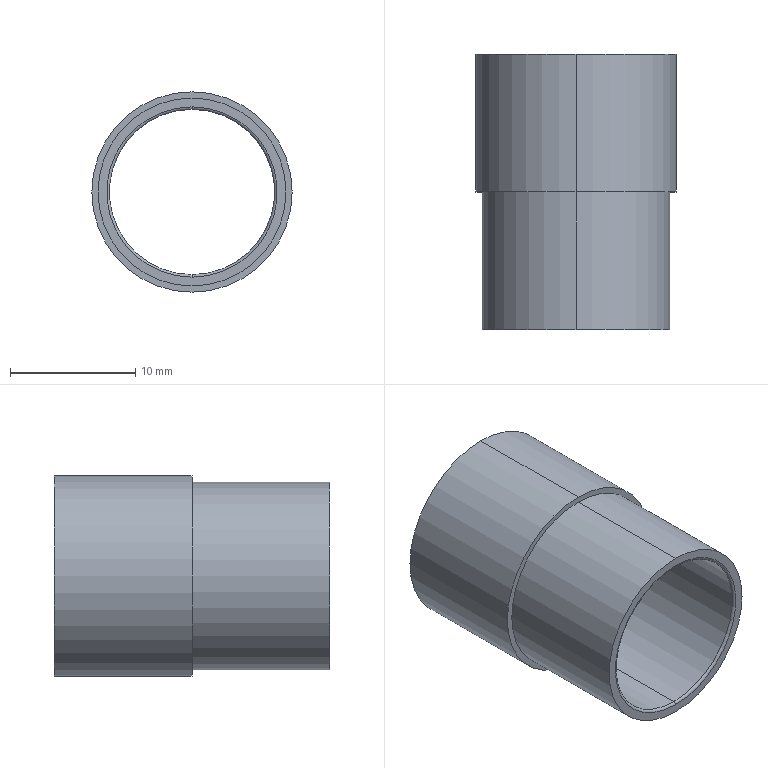Part | STEP file | G3L22N30-MM02TNNTNXH6-Part-1 | 1 solid | 11 faces | box 16 x 22 x 16 mm | volume 1145 mm3 | cylinder 6 | plane 3 | torus 2 | commonest cylinder face diameters 13.2 x2 15 x2 16 x2
STEP:
#1=CARTESIAN_POINT('',(-167.,-84.25,77.5));
#2=VERTEX_POINT('',#1);
#3=CARTESIAN_POINT('',(-167.,-84.25,93.5));
#4=VERTEX_POINT('',#3);
#5=CARTESIAN_POINT('',(-167.,-84.25,85.5));
#6=DIRECTION('',(0.,-1.,0.));
#7=DIRECTION('',(0.,0.,-1.));
#8=AXIS2_PLACEMENT_3D('',#5,#6,#7);
#9=CIRCLE('',#8,8.);
#10=EDGE_CURVE('',#2,#4,#9,.T.);
#11=ORIENTED_EDGE('',*,*,#10,.T.);
#12=CARTESIAN_POINT('',(-167.,-84.25,85.5));
#13=DIRECTION('',(0.,-1.,0.));
#14=DIRECTION('',(0.,0.,1.));
#15=AXIS2_PLACEMENT_3D('',#12,#13,#14);
#16=CIRCLE('',#15,8.);
#17=EDGE_CURVE('',#4,#2,#16,.T.);
#18=ORIENTED_EDGE('',*,*,#17,.T.);
#19=EDGE_LOOP('',(#11,#18));
#20=FACE_OUTER_BOUND('',#19,.T.);
#21=CARTESIAN_POINT('',(-167.,-84.25,78.));
#22=VERTEX_POINT('',#21);
#23=CARTESIAN_POINT('',(-167.,-84.25,93.));
#24=VERTEX_POINT('',#23);
#25=CARTESIAN_POINT('',(-167.,-84.25,85.5));
#26=DIRECTION('',(0.,-1.,0.));
#27=DIRECTION('',(0.,0.,-1.));
#28=AXIS2_PLACEMENT_3D('',#25,#26,#27);
#29=CIRCLE('',#28,7.5);
#30=EDGE_CURVE('',#22,#24,#29,.T.);
#31=ORIENTED_EDGE('',*,*,#30,.F.);
#32=CARTESIAN_POINT('',(-167.,-84.25,85.5));
#33=DIRECTION('',(0.,-1.,0.));
#34=DIRECTION('',(0.,0.,1.));
#35=AXIS2_PLACEMENT_3D('',#32,#33,#34);
#36=CIRCLE('',#35,7.5);
#37=EDGE_CURVE('',#24,#22,#36,.T.);
#38=ORIENTED_EDGE('',*,*,#37,.F.);
#39=EDGE_LOOP('',(#31,#38));
#40=FACE_BOUND('',#39,.T.);
#41=CARTESIAN_POINT('',(-183.971,-84.25,102.471));
#42=DIRECTION('',(0.,-1.,0.));
#43=DIRECTION('',(0.,0.,-1.));
#44=AXIS2_PLACEMENT_3D('',#41,#42,#43);
#45=PLANE('',#44);
#46=ADVANCED_FACE('',(#20,#40),#45,.T.);
#47=CARTESIAN_POINT('',(-167.,-73.25,77.5));
#48=VERTEX_POINT('',#47);
#49=CARTESIAN_POINT('',(-167.,-73.25,93.5));
#50=VERTEX_POINT('',#49);
#51=CARTESIAN_POINT('',(-167.,-73.25,85.5));
#52=DIRECTION('',(0.,-1.,0.));
#53=DIRECTION('',(0.,0.,-1.));
#54=AXIS2_PLACEMENT_3D('',#51,#52,#53);
#55=CIRCLE('',#54,8.);
#56=EDGE_CURVE('',#48,#50,#55,.T.);
#57=ORIENTED_EDGE('',*,*,#56,.T.);
#58=CARTESIAN_POINT('',(-167.,-73.25,93.5));
#59=DIRECTION('',(0.,-1.,0.));
#60=VECTOR('',#59,1000.);
#61=LINE('',#58,#60);
#62=EDGE_CURVE('',#50,#4,#61,.T.);
#63=ORIENTED_EDGE('',*,*,#62,.T.);
#64=ORIENTED_EDGE('',*,*,#10,.F.);
#65=CARTESIAN_POINT('',(-167.,-73.25,77.5));
#66=DIRECTION('',(0.,-1.,0.));
#67=VECTOR('',#66,1000.);
#68=LINE('',#65,#67);
#69=EDGE_CURVE('',#48,#2,#68,.T.);
#70=ORIENTED_EDGE('',*,*,#69,.F.);
#71=EDGE_LOOP('',(#57,#63,#64,#70));
#72=FACE_OUTER_BOUND('',#71,.T.);
#73=CARTESIAN_POINT('',(-167.,-78.75,85.5));
#74=DIRECTION('',(0.,-1.,0.));
#75=DIRECTION('',(0.,0.,-1.));
#76=AXIS2_PLACEMENT_3D('',#73,#74,#75);
#77=CYLINDRICAL_SURFACE('',#76,8.);
#78=ADVANCED_FACE('',(#72),#77,.T.);
#79=ORIENTED_EDGE('',*,*,#56,.F.);
#80=CARTESIAN_POINT('',(-167.,-73.25,85.5));
#81=DIRECTION('',(0.,-1.,0.));
#82=DIRECTION('',(0.,0.,1.));
#83=AXIS2_PLACEMENT_3D('',#80,#81,#82);
#84=CIRCLE('',#83,8.);
#85=EDGE_CURVE('',#50,#48,#84,.T.);
#86=ORIENTED_EDGE('',*,*,#85,.F.);
#87=EDGE_LOOP('',(#79,#86));
#88=FACE_OUTER_BOUND('',#87,.T.);
#89=CARTESIAN_POINT('',(-167.,-73.25,78.9));
#90=VERTEX_POINT('',#89);
#91=CARTESIAN_POINT('',(-167.,-73.25,92.1));
#92=VERTEX_POINT('',#91);
#93=CARTESIAN_POINT('',(-167.,-73.25,85.5));
#94=DIRECTION('',(0.,-1.,0.));
#95=DIRECTION('',(0.,0.,-1.));
#96=AXIS2_PLACEMENT_3D('',#93,#94,#95);
#97=CIRCLE('',#96,6.6);
#98=EDGE_CURVE('',#90,#92,#97,.T.);
#99=ORIENTED_EDGE('',*,*,#98,.T.);
#100=CARTESIAN_POINT('',(-167.,-73.25,85.5));
#101=DIRECTION('',(0.,-1.,0.));
#102=DIRECTION('',(0.,0.,1.));
#103=AXIS2_PLACEMENT_3D('',#100,#101,#102);
#104=CIRCLE('',#103,6.6);
#105=EDGE_CURVE('',#92,#90,#104,.T.);
#106=ORIENTED_EDGE('',*,*,#105,.T.);
#107=EDGE_LOOP('',(#99,#106));
#108=FACE_BOUND('',#107,.T.);
#109=CARTESIAN_POINT('',(-183.971,-73.25,102.471));
#110=DIRECTION('',(0.,-1.,0.));
#111=DIRECTION('',(0.,0.,-1.));
#112=AXIS2_PLACEMENT_3D('',#109,#110,#111);
#113=PLANE('',#112);
#114=ADVANCED_FACE('',(#88,#108),#113,.F.);
#115=CARTESIAN_POINT('',(-167.,-95.05,78.9));
#116=VERTEX_POINT('',#115);
#117=CARTESIAN_POINT('',(-167.,-95.05,92.1));
#118=VERTEX_POINT('',#117);
#119=CARTESIAN_POINT('',(-167.,-95.05,85.5));
#120=DIRECTION('',(0.,-1.,0.));
#121=DIRECTION('',(0.,0.,-1.));
#122=AXIS2_PLACEMENT_3D('',#119,#120,#121);
#123=CIRCLE('',#122,6.6);
#124=EDGE_CURVE('',#116,#118,#123,.T.);
#125=ORIENTED_EDGE('',*,*,#124,.T.);
#126=CARTESIAN_POINT('',(-167.,-73.25,92.1));
#127=DIRECTION('',(0.,-1.,0.));
#128=VECTOR('',#127,1000.);
#129=LINE('',#126,#128);
#130=EDGE_CURVE('',#92,#118,#129,.T.);
#131=ORIENTED_EDGE('',*,*,#130,.F.);
#132=ORIENTED_EDGE('',*,*,#98,.F.);
#133=CARTESIAN_POINT('',(-167.,-73.25,78.9));
#134=DIRECTION('',(0.,-1.,0.));
#135=VECTOR('',#134,1000.);
#136=LINE('',#133,#135);
#137=EDGE_CURVE('',#90,#116,#136,.T.);
#138=ORIENTED_EDGE('',*,*,#137,.T.);
#139=EDGE_LOOP('',(#125,#131,#132,#138));
#140=FACE_OUTER_BOUND('',#139,.T.);
#141=CARTESIAN_POINT('',(-167.,-84.15,85.5));
#142=DIRECTION('',(0.,-1.,0.));
#143=DIRECTION('',(0.,0.,-1.));
#144=AXIS2_PLACEMENT_3D('',#141,#142,#143);
#145=CYLINDRICAL_SURFACE('',#144,6.6);
#146=ADVANCED_FACE('',(#140),#145,.F.);
#147=CARTESIAN_POINT('',(-167.,-95.25,78.7));
#148=VERTEX_POINT('',#147);
#149=CARTESIAN_POINT('',(-167.,-95.25,92.3));
#150=VERTEX_POINT('',#149);
#151=CARTESIAN_POINT('',(-167.,-95.25,85.5));
#152=DIRECTION('',(0.,-1.,0.));
#153=DIRECTION('',(0.,0.,-1.));
#154=AXIS2_PLACEMENT_3D('',#151,#152,#153);
#155=CIRCLE('',#154,6.8);
#156=EDGE_CURVE('',#148,#150,#155,.T.);
#157=ORIENTED_EDGE('',*,*,#156,.T.);
#158=CARTESIAN_POINT('',(-167.,-95.05,92.3));
#159=DIRECTION('',(-1.,0.,0.));
#160=DIRECTION('',(0.,0.,-1.));
#161=AXIS2_PLACEMENT_3D('',#158,#159,#160);
#162=CIRCLE('',#161,0.2);
#163=EDGE_CURVE('',#118,#150,#162,.T.);
#164=ORIENTED_EDGE('',*,*,#163,.F.);
#165=ORIENTED_EDGE('',*,*,#124,.F.);
#166=CARTESIAN_POINT('',(-167.,-95.05,78.7));
#167=DIRECTION('',(1.,0.,0.));
#168=DIRECTION('',(0.,0.,1.));
#169=AXIS2_PLACEMENT_3D('',#166,#167,#168);
#170=CIRCLE('',#169,0.2);
#171=EDGE_CURVE('',#116,#148,#170,.T.);
#172=ORIENTED_EDGE('',*,*,#171,.T.);
#173=EDGE_LOOP('',(#157,#164,#165,#172));
#174=FACE_OUTER_BOUND('',#173,.T.);
#175=CARTESIAN_POINT('',(-167.,-95.05,85.5));
#176=DIRECTION('',(0.,-1.,0.));
#177=DIRECTION('',(0.,0.,1.));
#178=AXIS2_PLACEMENT_3D('',#175,#176,#177);
#179=TOROIDAL_SURFACE('',#178,6.8,0.2);
#180=ADVANCED_FACE('',(#174),#179,.T.);
#181=CARTESIAN_POINT('',(-167.,-95.25,78.));
#182=VERTEX_POINT('',#181);
#183=CARTESIAN_POINT('',(-167.,-95.25,93.));
#184=VERTEX_POINT('',#183);
#185=CARTESIAN_POINT('',(-167.,-95.25,85.5));
#186=DIRECTION('',(0.,-1.,0.));
#187=DIRECTION('',(0.,0.,-1.));
#188=AXIS2_PLACEMENT_3D('',#185,#186,#187);
#189=CIRCLE('',#188,7.5);
#190=EDGE_CURVE('',#182,#184,#189,.T.);
#191=ORIENTED_EDGE('',*,*,#190,.T.);
#192=CARTESIAN_POINT('',(-167.,-95.25,85.5));
#193=DIRECTION('',(0.,-1.,0.));
#194=DIRECTION('',(0.,0.,1.));
#195=AXIS2_PLACEMENT_3D('',#192,#193,#194);
#196=CIRCLE('',#195,7.5);
#197=EDGE_CURVE('',#184,#182,#196,.T.);
#198=ORIENTED_EDGE('',*,*,#197,.T.);
#199=EDGE_LOOP('',(#191,#198));
#200=FACE_OUTER_BOUND('',#199,.T.);
#201=ORIENTED_EDGE('',*,*,#156,.F.);
#202=CARTESIAN_POINT('',(-167.,-95.25,85.5));
#203=DIRECTION('',(0.,-1.,0.));
#204=DIRECTION('',(0.,0.,1.));
#205=AXIS2_PLACEMENT_3D('',#202,#203,#204);
#206=CIRCLE('',#205,6.8);
#207=EDGE_CURVE('',#150,#148,#206,.T.);
#208=ORIENTED_EDGE('',*,*,#207,.F.);
#209=EDGE_LOOP('',(#201,#208));
#210=FACE_BOUND('',#209,.T.);
#211=CARTESIAN_POINT('',(-182.91,-95.25,101.41));
#212=DIRECTION('',(0.,-1.,0.));
#213=DIRECTION('',(0.,0.,-1.));
#214=AXIS2_PLACEMENT_3D('',#211,#212,#213);
#215=PLANE('',#214);
#216=ADVANCED_FACE('',(#200,#210),#215,.T.);
#217=ORIENTED_EDGE('',*,*,#30,.T.);
#218=CARTESIAN_POINT('',(-167.,-84.25,93.));
#219=DIRECTION('',(0.,-1.,0.));
#220=VECTOR('',#219,1000.);
#221=LINE('',#218,#220);
#222=EDGE_CURVE('',#24,#184,#221,.T.);
#223=ORIENTED_EDGE('',*,*,#222,.T.);
#224=ORIENTED_EDGE('',*,*,#190,.F.);
#225=CARTESIAN_POINT('',(-167.,-84.25,78.));
#226=DIRECTION('',(0.,-1.,0.));
#227=VECTOR('',#226,1000.);
#228=LINE('',#225,#227);
#229=EDGE_CURVE('',#22,#182,#228,.T.);
#230=ORIENTED_EDGE('',*,*,#229,.F.);
#231=EDGE_LOOP('',(#217,#223,#224,#230));
#232=FACE_OUTER_BOUND('',#231,.T.);
#233=CARTESIAN_POINT('',(-167.,-89.75,85.5));
#234=DIRECTION('',(0.,-1.,0.));
#235=DIRECTION('',(0.,0.,-1.));
#236=AXIS2_PLACEMENT_3D('',#233,#234,#235);
#237=CYLINDRICAL_SURFACE('',#236,7.5);
#238=ADVANCED_FACE('',(#232),#237,.T.);
#239=ORIENTED_EDGE('',*,*,#137,.F.);
#240=ORIENTED_EDGE('',*,*,#105,.F.);
#241=ORIENTED_EDGE('',*,*,#130,.T.);
#242=CARTESIAN_POINT('',(-167.,-95.05,85.5));
#243=DIRECTION('',(0.,-1.,0.));
#244=DIRECTION('',(0.,0.,1.));
#245=AXIS2_PLACEMENT_3D('',#242,#243,#244);
#246=CIRCLE('',#245,6.6);
#247=EDGE_CURVE('',#118,#116,#246,.T.);
#248=ORIENTED_EDGE('',*,*,#247,.T.);
#249=EDGE_LOOP('',(#239,#240,#241,#248));
#250=FACE_OUTER_BOUND('',#249,.T.);
#251=CARTESIAN_POINT('',(-167.,-84.15,85.5));
#252=DIRECTION('',(0.,-1.,0.));
#253=DIRECTION('',(0.,0.,-1.));
#254=AXIS2_PLACEMENT_3D('',#251,#252,#253);
#255=CYLINDRICAL_SURFACE('',#254,6.6);
#256=ADVANCED_FACE('',(#250),#255,.F.);
#257=ORIENTED_EDGE('',*,*,#229,.T.);
#258=ORIENTED_EDGE('',*,*,#197,.F.);
#259=ORIENTED_EDGE('',*,*,#222,.F.);
#260=ORIENTED_EDGE('',*,*,#37,.T.);
#261=EDGE_LOOP('',(#257,#258,#259,#260));
#262=FACE_OUTER_BOUND('',#261,.T.);
#263=CARTESIAN_POINT('',(-167.,-89.75,85.5));
#264=DIRECTION('',(0.,-1.,0.));
#265=DIRECTION('',(0.,0.,-1.));
#266=AXIS2_PLACEMENT_3D('',#263,#264,#265);
#267=CYLINDRICAL_SURFACE('',#266,7.5);
#268=ADVANCED_FACE('',(#262),#267,.T.);
#269=ORIENTED_EDGE('',*,*,#69,.T.);
#270=ORIENTED_EDGE('',*,*,#17,.F.);
#271=ORIENTED_EDGE('',*,*,#62,.F.);
#272=ORIENTED_EDGE('',*,*,#85,.T.);
#273=EDGE_LOOP('',(#269,#270,#271,#272));
#274=FACE_OUTER_BOUND('',#273,.T.);
#275=CARTESIAN_POINT('',(-167.,-78.75,85.5));
#276=DIRECTION('',(0.,-1.,0.));
#277=DIRECTION('',(0.,0.,-1.));
#278=AXIS2_PLACEMENT_3D('',#275,#276,#277);
#279=CYLINDRICAL_SURFACE('',#278,8.);
#280=ADVANCED_FACE('',(#274),#279,.T.);
#281=ORIENTED_EDGE('',*,*,#163,.T.);
#282=ORIENTED_EDGE('',*,*,#207,.T.);
#283=ORIENTED_EDGE('',*,*,#171,.F.);
#284=ORIENTED_EDGE('',*,*,#247,.F.);
#285=EDGE_LOOP('',(#281,#282,#283,#284));
#286=FACE_OUTER_BOUND('',#285,.T.);
#287=CARTESIAN_POINT('',(-167.,-95.05,85.5));
#288=DIRECTION('',(0.,-1.,0.));
#289=DIRECTION('',(0.,0.,1.));
#290=AXIS2_PLACEMENT_3D('',#287,#288,#289);
#291=TOROIDAL_SURFACE('',#290,6.8,0.2);
#292=ADVANCED_FACE('',(#286),#291,.T.);
#293=CLOSED_SHELL('',(#46,#78,#114,#146,#180,#216,#238,#256,#268,#280,#292));
#294=MANIFOLD_SOLID_BREP('',#293);
#295=CARTESIAN_POINT('',(0.,0.,0.));
#296=DIRECTION('',(0.,0.,1.));
#297=DIRECTION('',(1.,0.,0.));
#298=AXIS2_PLACEMENT_3D('',#295,#296,#297);
#299=(LENGTH_UNIT()NAMED_UNIT(*)SI_UNIT(.MILLI.,.METRE.));
#300=UNCERTAINTY_MEASURE_WITH_UNIT(LENGTH_MEASURE(0.00001),#299,'','');
#301=(NAMED_UNIT(*)PLANE_ANGLE_UNIT()SI_UNIT($,.RADIAN.));
#302=(NAMED_UNIT(*)SI_UNIT($,.STERADIAN.)SOLID_ANGLE_UNIT());
#303=(GEOMETRIC_REPRESENTATION_CONTEXT(3)GLOBAL_UNCERTAINTY_ASSIGNED_CONTEXT((#300))GLOBAL_UNIT_ASSIGNED_CONTEXT((#299,#301,#302))REPRESENTATION_CONTEXT('',''));
#304=ADVANCED_BREP_SHAPE_REPRESENTATION('',(#294,#298),#303);